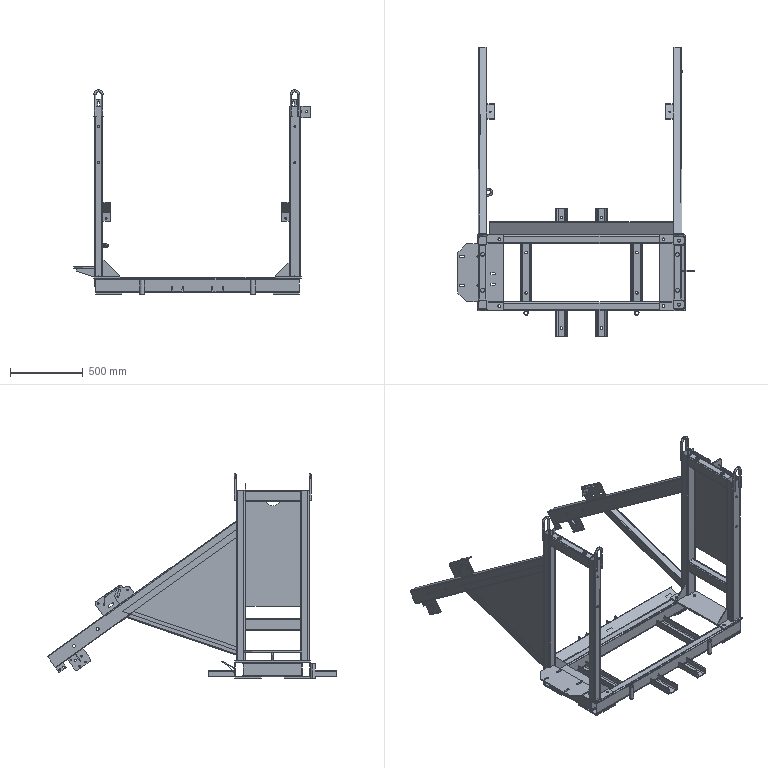Part | SolidWorks | features CompositeCurve 16 | 62 solids | 1063 faces | box 1625 x 1990 x 1408 mm | volume 21000923 mm3 | plane 567 | cylinder 450 | cone 26 | torus 20 | commonest cylinder face diameters 12 x74 18 x64 14 x48 16 x42 8 x40 20 x39